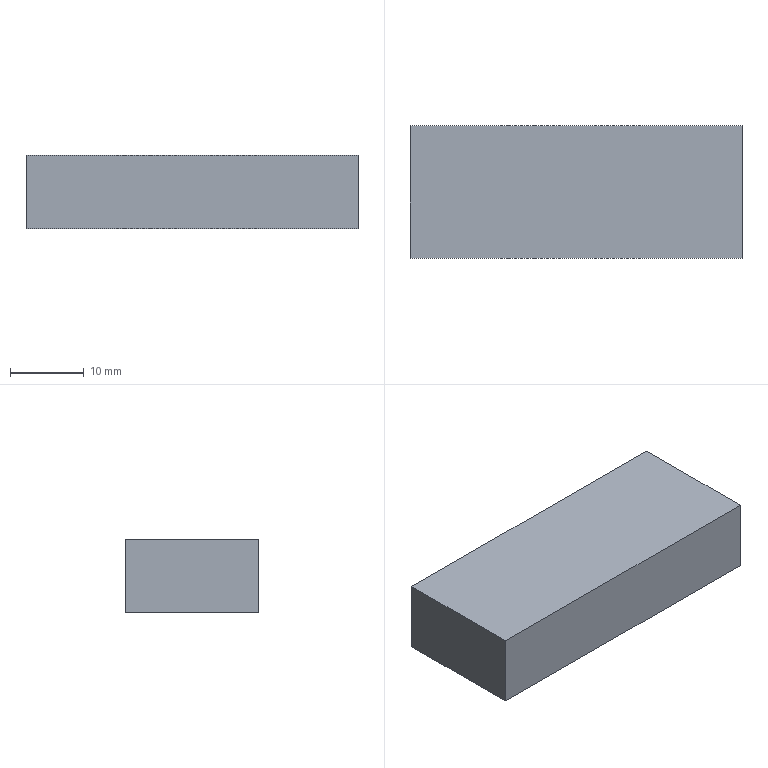Part | SolidWorks | features Extrusion 1 | 1 solid | 6 faces | box 45 x 18 x 10 mm | volume 8100 mm3 | plane 6
STEP:
#1=CARTESIAN_POINT('',(-22.5,9.,5.));
#2=VERTEX_POINT('',#1);
#3=CARTESIAN_POINT('',(-22.5,-9.,5.));
#4=VERTEX_POINT('',#3);
#5=CARTESIAN_POINT('',(-22.5,9.,5.));
#6=DIRECTION('',(0.,-1.,0.));
#7=VECTOR('',#6,1000.);
#8=LINE('',#5,#7);
#9=EDGE_CURVE('',#2,#4,#8,.T.);
#10=ORIENTED_EDGE('',*,*,#9,.F.);
#11=CARTESIAN_POINT('',(-22.5,9.,-5.));
#12=VERTEX_POINT('',#11);
#13=CARTESIAN_POINT('',(-22.5,9.,-5.));
#14=DIRECTION('',(0.,0.,1.));
#15=VECTOR('',#14,1000.);
#16=LINE('',#13,#15);
#17=EDGE_CURVE('',#12,#2,#16,.T.);
#18=ORIENTED_EDGE('',*,*,#17,.F.);
#19=CARTESIAN_POINT('',(-22.5,-9.,-5.));
#20=VERTEX_POINT('',#19);
#21=CARTESIAN_POINT('',(-22.5,9.,-5.));
#22=DIRECTION('',(0.,-1.,0.));
#23=VECTOR('',#22,1000.);
#24=LINE('',#21,#23);
#25=EDGE_CURVE('',#12,#20,#24,.T.);
#26=ORIENTED_EDGE('',*,*,#25,.T.);
#27=CARTESIAN_POINT('',(-22.5,-9.,-5.));
#28=DIRECTION('',(0.,0.,1.));
#29=VECTOR('',#28,1000.);
#30=LINE('',#27,#29);
#31=EDGE_CURVE('',#20,#4,#30,.T.);
#32=ORIENTED_EDGE('',*,*,#31,.T.);
#33=EDGE_LOOP('',(#10,#18,#26,#32));
#34=FACE_OUTER_BOUND('',#33,.T.);
#35=CARTESIAN_POINT('',(-22.5,9.,-5.));
#36=DIRECTION('',(-1.,0.,0.));
#37=DIRECTION('',(0.,0.,1.));
#38=AXIS2_PLACEMENT_3D('',#35,#36,#37);
#39=PLANE('',#38);
#40=ADVANCED_FACE('',(#34),#39,.T.);
#41=CARTESIAN_POINT('',(22.5,9.,5.));
#42=VERTEX_POINT('',#41);
#43=CARTESIAN_POINT('',(22.5,9.,5.));
#44=DIRECTION('',(-1.,0.,0.));
#45=VECTOR('',#44,1000.);
#46=LINE('',#43,#45);
#47=EDGE_CURVE('',#42,#2,#46,.T.);
#48=ORIENTED_EDGE('',*,*,#47,.F.);
#49=CARTESIAN_POINT('',(22.5,9.,-5.));
#50=VERTEX_POINT('',#49);
#51=CARTESIAN_POINT('',(22.5,9.,-5.));
#52=DIRECTION('',(0.,0.,1.));
#53=VECTOR('',#52,1000.);
#54=LINE('',#51,#53);
#55=EDGE_CURVE('',#50,#42,#54,.T.);
#56=ORIENTED_EDGE('',*,*,#55,.F.);
#57=CARTESIAN_POINT('',(22.5,9.,-5.));
#58=DIRECTION('',(-1.,0.,0.));
#59=VECTOR('',#58,1000.);
#60=LINE('',#57,#59);
#61=EDGE_CURVE('',#50,#12,#60,.T.);
#62=ORIENTED_EDGE('',*,*,#61,.T.);
#63=ORIENTED_EDGE('',*,*,#17,.T.);
#64=EDGE_LOOP('',(#48,#56,#62,#63));
#65=FACE_OUTER_BOUND('',#64,.T.);
#66=CARTESIAN_POINT('',(22.5,9.,-5.));
#67=DIRECTION('',(0.,1.,0.));
#68=DIRECTION('',(0.,0.,1.));
#69=AXIS2_PLACEMENT_3D('',#66,#67,#68);
#70=PLANE('',#69);
#71=ADVANCED_FACE('',(#65),#70,.T.);
#72=CARTESIAN_POINT('',(22.5,-9.,5.));
#73=VERTEX_POINT('',#72);
#74=CARTESIAN_POINT('',(22.5,-9.,5.));
#75=DIRECTION('',(0.,1.,0.));
#76=VECTOR('',#75,1000.);
#77=LINE('',#74,#76);
#78=EDGE_CURVE('',#73,#42,#77,.T.);
#79=ORIENTED_EDGE('',*,*,#78,.F.);
#80=CARTESIAN_POINT('',(22.5,-9.,-5.));
#81=VERTEX_POINT('',#80);
#82=CARTESIAN_POINT('',(22.5,-9.,-5.));
#83=DIRECTION('',(0.,0.,1.));
#84=VECTOR('',#83,1000.);
#85=LINE('',#82,#84);
#86=EDGE_CURVE('',#81,#73,#85,.T.);
#87=ORIENTED_EDGE('',*,*,#86,.F.);
#88=CARTESIAN_POINT('',(22.5,-9.,-5.));
#89=DIRECTION('',(0.,1.,0.));
#90=VECTOR('',#89,1000.);
#91=LINE('',#88,#90);
#92=EDGE_CURVE('',#81,#50,#91,.T.);
#93=ORIENTED_EDGE('',*,*,#92,.T.);
#94=ORIENTED_EDGE('',*,*,#55,.T.);
#95=EDGE_LOOP('',(#79,#87,#93,#94));
#96=FACE_OUTER_BOUND('',#95,.T.);
#97=CARTESIAN_POINT('',(22.5,-9.,-5.));
#98=DIRECTION('',(1.,0.,0.));
#99=DIRECTION('',(0.,0.,-1.));
#100=AXIS2_PLACEMENT_3D('',#97,#98,#99);
#101=PLANE('',#100);
#102=ADVANCED_FACE('',(#96),#101,.T.);
#103=CARTESIAN_POINT('',(-22.5,-9.,5.));
#104=DIRECTION('',(1.,0.,0.));
#105=VECTOR('',#104,1000.);
#106=LINE('',#103,#105);
#107=EDGE_CURVE('',#4,#73,#106,.T.);
#108=ORIENTED_EDGE('',*,*,#107,.F.);
#109=ORIENTED_EDGE('',*,*,#31,.F.);
#110=CARTESIAN_POINT('',(-22.5,-9.,-5.));
#111=DIRECTION('',(1.,0.,0.));
#112=VECTOR('',#111,1000.);
#113=LINE('',#110,#112);
#114=EDGE_CURVE('',#20,#81,#113,.T.);
#115=ORIENTED_EDGE('',*,*,#114,.T.);
#116=ORIENTED_EDGE('',*,*,#86,.T.);
#117=EDGE_LOOP('',(#108,#109,#115,#116));
#118=FACE_OUTER_BOUND('',#117,.T.);
#119=CARTESIAN_POINT('',(-22.5,-9.,-5.));
#120=DIRECTION('',(0.,-1.,0.));
#121=DIRECTION('',(0.,0.,-1.));
#122=AXIS2_PLACEMENT_3D('',#119,#120,#121);
#123=PLANE('',#122);
#124=ADVANCED_FACE('',(#118),#123,.T.);
#125=ORIENTED_EDGE('',*,*,#25,.F.);
#126=ORIENTED_EDGE('',*,*,#61,.F.);
#127=ORIENTED_EDGE('',*,*,#92,.F.);
#128=ORIENTED_EDGE('',*,*,#114,.F.);
#129=EDGE_LOOP('',(#125,#126,#127,#128));
#130=FACE_OUTER_BOUND('',#129,.T.);
#131=CARTESIAN_POINT('',(0.,0.,-5.));
#132=DIRECTION('',(0.,0.,1.));
#133=DIRECTION('',(1.,0.,0.));
#134=AXIS2_PLACEMENT_3D('',#131,#132,#133);
#135=PLANE('',#134);
#136=ADVANCED_FACE('',(#130),#135,.F.);
#137=ORIENTED_EDGE('',*,*,#9,.T.);
#138=ORIENTED_EDGE('',*,*,#107,.T.);
#139=ORIENTED_EDGE('',*,*,#78,.T.);
#140=ORIENTED_EDGE('',*,*,#47,.T.);
#141=EDGE_LOOP('',(#137,#138,#139,#140));
#142=FACE_OUTER_BOUND('',#141,.T.);
#143=CARTESIAN_POINT('',(0.,0.,5.));
#144=DIRECTION('',(0.,0.,1.));
#145=DIRECTION('',(1.,0.,0.));
#146=AXIS2_PLACEMENT_3D('',#143,#144,#145);
#147=PLANE('',#146);
#148=ADVANCED_FACE('',(#142),#147,.T.);
#149=CLOSED_SHELL('',(#40,#71,#102,#124,#136,#148));
#150=MANIFOLD_SOLID_BREP('',#149);
#151=CARTESIAN_POINT('',(0.,0.,0.));
#152=DIRECTION('',(0.,0.,1.));
#153=DIRECTION('',(1.,0.,0.));
#154=AXIS2_PLACEMENT_3D('',#151,#152,#153);
#155=(LENGTH_UNIT()NAMED_UNIT(*)SI_UNIT(.MILLI.,.METRE.));
#156=UNCERTAINTY_MEASURE_WITH_UNIT(LENGTH_MEASURE(0.00001),#155,'','');
#157=(NAMED_UNIT(*)PLANE_ANGLE_UNIT()SI_UNIT($,.RADIAN.));
#158=(NAMED_UNIT(*)SI_UNIT($,.STERADIAN.)SOLID_ANGLE_UNIT());
#159=(GEOMETRIC_REPRESENTATION_CONTEXT(3)GLOBAL_UNCERTAINTY_ASSIGNED_CONTEXT((#156))GLOBAL_UNIT_ASSIGNED_CONTEXT((#155,#157,#158))REPRESENTATION_CONTEXT('',''));
#160=ADVANCED_BREP_SHAPE_REPRESENTATION('',(#150,#154),#159);